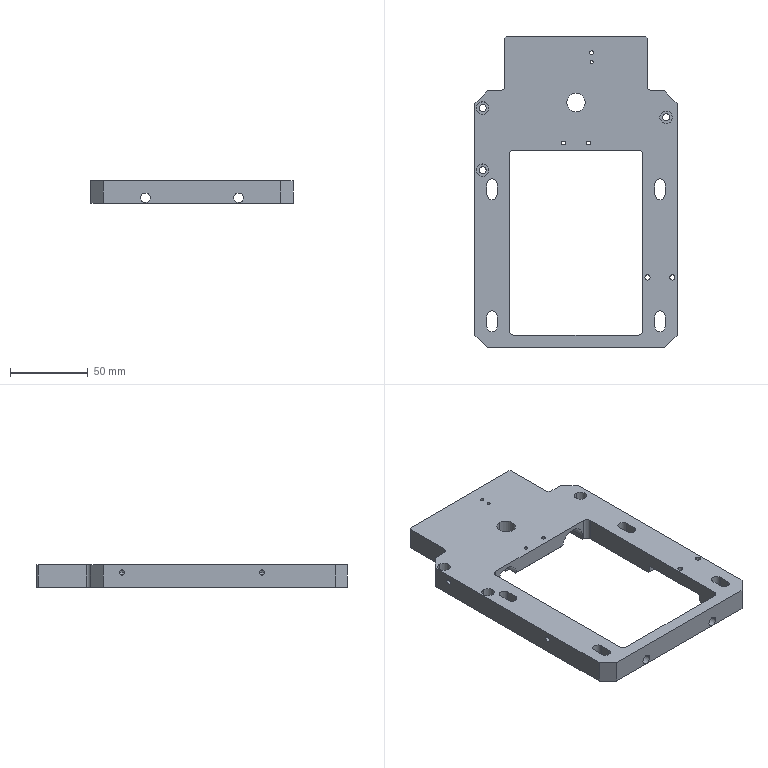NC program | NX | posted with a generic post | part box 130 x 200 x 14.5 mm
Lines 6565 to 7418 of 25347:
(ZLEVEL_PROFILE_1_COPY_1 , TOOL : D6)
N13062 T06 M6
N13064 G54
N13066 G17 G0 G90 X-88.086 Y-55.995 B0. C0. S4000 M3
N13068 G43 Z30. H6
N13070 Z1.5
N13072 G94 G1 X-88.016 Y-56.051 Z1.495 F1000.
N13074 X-87.513 Y-56.286 Z1.466
N13076 X-86.969 Y-56.4 Z1.437
N13078 X-79.531 Z1.047
N13080 X-79.017 Y-56.296 Z1.02
N13082 X-78.537 Y-56.083 Z0.992
N13084 X-78.115 Y-55.771 Z0.965
N13086 X-77.771 Y-55.375 Z0.937
N13088 X-77.52 Y-54.914 Z0.91
N13090 X-77.391 Y-54.495 Z0.887
N13092 X-77.341 Y-53.918 Z0.856
N13094 X-77.431 Y-53.346 Z0.826
N13096 X-77.654 Y-52.811 Z0.796
N13098 X-77.998 Y-52.345 Z0.765
N13100 X-78.443 Y-51.975 Z0.735
N13102 X-78.964 Y-51.722 Z0.705
N13104 X-79.531 Y-51.6 Z0.674
N13106 X-86.969 Z0.284
N13108 X-87.515 Y-51.715 Z0.255
N13110 X-88.019 Y-51.951 Z0.226
N13112 X-88.456 Y-52.298 Z0.197
N13114 X-88.801 Y-52.735 Z0.168
N13116 X-89.037 Y-53.24 Z0.138
N13118 X-89.15 Y-53.786 Z0.109
N13120 X-89.149 Y-54.225 Z0.086
N13122 X-89.034 Y-54.768 Z0.057
N13124 X-88.798 Y-55.271 Z0.028
N13126 X-88.452 Y-55.706 Z-0.001
N13128 X-88.016 Y-56.051 Z-0.03
N13130 X-87.513 Y-56.286 Z-0.059
N13132 X-86.969 Y-56.4 Z-0.089
N13134 X-86.75 Z-0.1
N13136 X-79.75 F1800.
N13138 G3 X-77.35 Y-54. R2.4
N13140 X-79.75 Y-51.6 R2.4
N13142 G1 X-86.75
N13144 G3 X-89.15 Y-54. R2.4
N13146 X-86.75 Y-56.4 R2.4
N13148 G1 X-82.538 Z-0.174
N13150 X-82.369 Y-56.399 Z-0.176
N13152 X-82.201 Y-56.4 Z-0.179
N13154 X-82.032 Y-56.399 Z-0.182
N13156 X-81.864 Y-56.4 Z-0.185
N13158 X-81.695 Y-56.399 Z-0.188
N13160 X-81.527 Y-56.4 Z-0.191
N13162 X-81.358 Y-56.399 Z-0.194
N13164 X-81.19 Y-56.4 Z-0.197
N13166 X-81.021 Z-0.2
N13168 X-79.75
N13170 G3 X-77.35 Y-54. R2.4
N13172 X-79.75 Y-51.6 R2.4
N13174 G1 X-86.75
N13176 G3 X-89.15 Y-54. R2.4
N13178 X-86.75 Y-56.4 R2.4
N13180 G1 X-82.538 Z-0.274
N13182 X-82.369 Y-56.399 Z-0.276
N13184 X-82.201 Y-56.4 Z-0.279
N13186 X-82.032 Y-56.399 Z-0.282
N13188 X-81.864 Y-56.4 Z-0.285
N13190 X-81.695 Y-56.399 Z-0.288
N13192 X-81.527 Y-56.4 Z-0.291
N13194 X-81.358 Y-56.399 Z-0.294
N13196 X-81.19 Y-56.4 Z-0.297
N13198 X-81.021 Z-0.3
N13200 X-79.75
N13202 G3 X-77.35 Y-54. R2.4
N13204 X-79.75 Y-51.6 R2.4
N13206 G1 X-86.75
N13208 G3 X-89.15 Y-54. R2.4
N13210 X-86.75 Y-56.4 R2.4
N13212 G1 X-82.538 Z-0.374
N13214 X-82.369 Y-56.399 Z-0.376
N13216 X-82.201 Y-56.4 Z-0.379
N13218 X-82.032 Y-56.399 Z-0.382
N13220 X-81.864 Y-56.4 Z-0.385
N13222 X-81.695 Y-56.399 Z-0.388
N13224 X-81.527 Y-56.4 Z-0.391
N13226 X-81.358 Y-56.399 Z-0.394
N13228 X-81.19 Y-56.4 Z-0.397
N13230 X-81.021 Z-0.4
N13232 X-79.75
N13234 G3 X-77.35 Y-54. R2.4
N13236 X-79.75 Y-51.6 R2.4
N13238 G1 X-86.75
N13240 G3 X-89.15 Y-54. R2.4
N13242 X-86.75 Y-56.4 R2.4
N13244 G1 X-82.538 Z-0.474
N13246 X-82.369 Y-56.399 Z-0.476
N13248 X-82.201 Y-56.4 Z-0.479
N13250 X-82.032 Y-56.399 Z-0.482
N13252 X-81.864 Y-56.4 Z-0.485
N13254 X-81.695 Y-56.399 Z-0.488
N13256 X-81.527 Y-56.4 Z-0.491
N13258 X-81.358 Y-56.399 Z-0.494
N13260 X-81.19 Y-56.4 Z-0.497
N13262 X-81.021 Z-0.5
N13264 X-79.75
N13266 G3 X-77.35 Y-54. R2.4
N13268 X-79.75 Y-51.6 R2.4
N13270 G1 X-86.75
N13272 G3 X-89.15 Y-54. R2.4
N13274 X-86.75 Y-56.4 R2.4
N13276 G1 X-82.538 Z-0.574
N13278 X-82.369 Y-56.399 Z-0.576
N13280 X-82.201 Y-56.4 Z-0.579
N13282 X-82.032 Y-56.399 Z-0.582
N13284 X-81.864 Y-56.4 Z-0.585
N13286 X-81.695 Y-56.399 Z-0.588
N13288 X-81.527 Y-56.4 Z-0.591
N13290 X-81.358 Y-56.399 Z-0.594
N13292 X-81.19 Y-56.4 Z-0.597
N13294 X-81.021 Z-0.6
N13296 X-79.75
N13298 G3 X-77.35 Y-54. R2.4
N13300 X-79.75 Y-51.6 R2.4
N13302 G1 X-86.75
N13304 G3 X-89.15 Y-54. R2.4
N13306 X-86.75 Y-56.4 R2.4
N13308 G1 X-82.538 Z-0.674
N13310 X-82.369 Y-56.399 Z-0.676
N13312 X-82.201 Y-56.4 Z-0.679
N13314 X-82.032 Y-56.399 Z-0.682
N13316 X-81.864 Y-56.4 Z-0.685
N13318 X-81.695 Y-56.399 Z-0.688
N13320 X-81.527 Y-56.4 Z-0.691
N13322 X-81.358 Y-56.399 Z-0.694
N13324 X-81.19 Y-56.4 Z-0.697
N13326 X-81.021 Z-0.7
N13328 X-79.75
N13330 G3 X-77.35 Y-54. R2.4
N13332 X-79.75 Y-51.6 R2.4
N13334 G1 X-86.75
N13336 G3 X-89.15 Y-54. R2.4
N13338 X-86.75 Y-56.4 R2.4
N13340 G1 X-82.538 Z-0.774
N13342 X-82.369 Y-56.399 Z-0.776
N13344 X-82.201 Y-56.4 Z-0.779
N13346 X-82.032 Y-56.399 Z-0.782
N13348 X-81.864 Y-56.4 Z-0.785
N13350 X-81.695 Y-56.399 Z-0.788
N13352 X-81.527 Y-56.4 Z-0.791
N13354 X-81.358 Y-56.399 Z-0.794
N13356 X-81.19 Y-56.4 Z-0.797
N13358 X-81.021 Z-0.8
N13360 X-79.75
N13362 G3 X-77.35 Y-54. R2.4
N13364 X-79.75 Y-51.6 R2.4
N13366 G1 X-86.75
N13368 G3 X-89.15 Y-54. R2.4
N13370 X-86.75 Y-56.4 R2.4
N13372 G1 X-82.538 Z-0.874
N13374 X-82.369 Y-56.399 Z-0.876
N13376 X-82.201 Y-56.4 Z-0.879
N13378 X-82.032 Y-56.399 Z-0.882
N13380 X-81.864 Y-56.4 Z-0.885
N13382 X-81.695 Y-56.399 Z-0.888
N13384 X-81.527 Y-56.4 Z-0.891
N13386 X-81.358 Y-56.399 Z-0.894
N13388 X-81.19 Y-56.4 Z-0.897
N13390 X-81.021 Z-0.9
N13392 X-79.75
N13394 G3 X-77.35 Y-54. R2.4
N13396 X-79.75 Y-51.6 R2.4
N13398 G1 X-86.75
N13400 G3 X-89.15 Y-54. R2.4
N13402 X-86.75 Y-56.4 R2.4
N13404 G1 X-82.538 Z-0.974
N13406 X-82.369 Y-56.399 Z-0.976
N13408 X-82.201 Y-56.4 Z-0.979
N13410 X-82.032 Y-56.399 Z-0.982
N13412 X-81.864 Y-56.4 Z-0.985
N13414 X-81.695 Y-56.399 Z-0.988
N13416 X-81.527 Y-56.4 Z-0.991
N13418 X-81.358 Y-56.399 Z-0.994
N13420 X-81.19 Y-56.4 Z-0.997
N13422 X-81.021 Z-1.
N13424 X-79.75
N13426 G3 X-77.35 Y-54. R2.4
N13428 X-79.75 Y-51.6 R2.4
N13430 G1 X-86.75
N13432 G3 X-89.15 Y-54. R2.4
N13434 X-86.75 Y-56.4 R2.4
N13436 G1 X-82.538 Z-1.074
N13438 X-82.369 Y-56.399 Z-1.076
N13440 X-82.201 Y-56.4 Z-1.079
N13442 X-82.032 Y-56.399 Z-1.082
N13444 X-81.864 Y-56.4 Z-1.085
N13446 X-81.695 Y-56.399 Z-1.088
N13448 X-81.527 Y-56.4 Z-1.091
N13450 X-81.358 Y-56.399 Z-1.094
N13452 X-81.19 Y-56.4 Z-1.097
N13454 X-81.021 Z-1.1
N13456 X-79.75
N13458 G3 X-77.35 Y-54. R2.4
N13460 X-79.75 Y-51.6 R2.4
N13462 G1 X-86.75
N13464 G3 X-89.15 Y-54. R2.4
N13466 X-86.75 Y-56.4 R2.4
N13468 G1 X-82.538 Z-1.174
N13470 X-82.369 Y-56.399 Z-1.176
N13472 X-82.201 Y-56.4 Z-1.179
N13474 X-82.032 Y-56.399 Z-1.182
N13476 X-81.864 Y-56.4 Z-1.185
N13478 X-81.695 Y-56.399 Z-1.188
N13480 X-81.527 Y-56.4 Z-1.191
N13482 X-81.358 Y-56.399 Z-1.194
N13484 X-81.19 Y-56.4 Z-1.197
N13486 X-81.021 Z-1.2
N13488 X-79.75
N13490 G3 X-77.35 Y-54. R2.4
N13492 X-79.75 Y-51.6 R2.4
N13494 G1 X-86.75
N13496 G3 X-89.15 Y-54. R2.4
N13498 X-86.75 Y-56.4 R2.4
N13500 G1 X-82.538 Z-1.274
N13502 X-82.369 Y-56.399 Z-1.276
N13504 X-82.201 Y-56.4 Z-1.279
N13506 X-82.032 Y-56.399 Z-1.282
N13508 X-81.864 Y-56.4 Z-1.285
N13510 X-81.695 Y-56.399 Z-1.288
N13512 X-81.527 Y-56.4 Z-1.291
N13514 X-81.358 Y-56.399 Z-1.294
N13516 X-81.19 Y-56.4 Z-1.297
N13518 X-81.021 Z-1.3
N13520 X-79.75
N13522 G3 X-77.35 Y-54. R2.4
N13524 X-79.75 Y-51.6 R2.4
N13526 G1 X-86.75
N13528 G3 X-89.15 Y-54. R2.4
N13530 X-86.75 Y-56.4 R2.4
N13532 G1 X-82.538 Z-1.374
N13534 X-82.369 Y-56.399 Z-1.376
N13536 X-82.201 Y-56.4 Z-1.379
N13538 X-82.032 Y-56.399 Z-1.382
N13540 X-81.864 Y-56.4 Z-1.385
N13542 X-81.695 Y-56.399 Z-1.388
N13544 X-81.527 Y-56.4 Z-1.391
N13546 X-81.358 Y-56.399 Z-1.394
N13548 X-81.19 Y-56.4 Z-1.397
N13550 X-81.021 Z-1.4
N13552 X-79.75
N13554 G3 X-77.35 Y-54. R2.4
N13556 X-79.75 Y-51.6 R2.4
N13558 G1 X-86.75
N13560 G3 X-89.15 Y-54. R2.4
N13562 X-86.75 Y-56.4 R2.4
N13564 G1 X-82.538 Z-1.474
N13566 X-82.369 Y-56.399 Z-1.476
N13568 X-82.201 Y-56.4 Z-1.479
N13570 X-82.032 Y-56.399 Z-1.482
N13572 X-81.864 Y-56.4 Z-1.485
N13574 X-81.695 Y-56.399 Z-1.488
N13576 X-81.527 Y-56.4 Z-1.491
N13578 X-81.358 Y-56.399 Z-1.494
N13580 X-81.19 Y-56.4 Z-1.497
N13582 X-81.021 Z-1.5
N13584 X-79.75
N13586 G3 X-77.35 Y-54. R2.4
N13588 X-79.75 Y-51.6 R2.4
N13590 G1 X-86.75
N13592 G3 X-89.15 Y-54. R2.4
N13594 X-86.75 Y-56.4 R2.4
N13596 G1 X-82.538 Z-1.574
N13598 X-82.369 Y-56.399 Z-1.576
N13600 X-82.201 Y-56.4 Z-1.579
N13602 X-82.032 Y-56.399 Z-1.582
N13604 X-81.864 Y-56.4 Z-1.585
N13606 X-81.695 Y-56.399 Z-1.588
N13608 X-81.527 Y-56.4 Z-1.591
N13610 X-81.358 Y-56.399 Z-1.594
N13612 X-81.19 Y-56.4 Z-1.597
N13614 X-81.021 Z-1.6
N13616 X-79.75
N13618 G3 X-77.35 Y-54. R2.4
N13620 X-79.75 Y-51.6 R2.4
N13622 G1 X-86.75
N13624 G3 X-89.15 Y-54. R2.4
N13626 X-86.75 Y-56.4 R2.4
N13628 G1 X-82.538 Z-1.674
N13630 X-82.369 Y-56.399 Z-1.676
N13632 X-82.201 Y-56.4 Z-1.679
N13634 X-82.032 Y-56.399 Z-1.682
N13636 X-81.864 Y-56.4 Z-1.685
N13638 X-81.695 Y-56.399 Z-1.688
N13640 X-81.527 Y-56.4 Z-1.691
N13642 X-81.358 Y-56.399 Z-1.694
N13644 X-81.19 Y-56.4 Z-1.697
N13646 X-81.021 Z-1.7
N13648 X-79.75
N13650 G3 X-77.35 Y-54. R2.4
N13652 X-79.75 Y-51.6 R2.4
N13654 G1 X-86.75
N13656 G3 X-89.15 Y-54. R2.4
N13658 X-86.75 Y-56.4 R2.4
N13660 G1 X-82.538 Z-1.774
N13662 X-82.369 Y-56.399 Z-1.776
N13664 X-82.201 Y-56.4 Z-1.779
N13666 X-82.032 Y-56.399 Z-1.782
N13668 X-81.864 Y-56.4 Z-1.785
N13670 X-81.695 Y-56.399 Z-1.788
N13672 X-81.527 Y-56.4 Z-1.791
N13674 X-81.358 Y-56.399 Z-1.794
N13676 X-81.19 Y-56.4 Z-1.797
N13678 X-81.021 Z-1.8
N13680 X-79.75
N13682 G3 X-77.35 Y-54. R2.4
N13684 X-79.75 Y-51.6 R2.4
N13686 G1 X-86.75
N13688 G3 X-89.15 Y-54. R2.4
N13690 X-86.75 Y-56.4 R2.4
N13692 G1 X-82.538 Z-1.874
N13694 X-82.369 Y-56.399 Z-1.876
N13696 X-82.201 Y-56.4 Z-1.879
N13698 X-82.032 Y-56.399 Z-1.882
N13700 X-81.864 Y-56.4 Z-1.885
N13702 X-81.695 Y-56.399 Z-1.888
N13704 X-81.527 Y-56.4 Z-1.891
N13706 X-81.358 Y-56.399 Z-1.894
N13708 X-81.19 Y-56.4 Z-1.897
N13710 X-81.021 Z-1.9
N13712 X-79.75
N13714 G3 X-77.35 Y-54. R2.4
N13716 X-79.75 Y-51.6 R2.4
N13718 G1 X-86.75
N13720 G3 X-89.15 Y-54. R2.4
N13722 X-86.75 Y-56.4 R2.4
N13724 G1 X-82.538 Z-1.974
N13726 X-82.369 Y-56.399 Z-1.976
N13728 X-82.201 Y-56.4 Z-1.979
N13730 X-82.032 Y-56.399 Z-1.982
N13732 X-81.864 Y-56.4 Z-1.985
N13734 X-81.695 Y-56.399 Z-1.988
N13736 X-81.527 Y-56.4 Z-1.991
N13738 X-81.358 Y-56.399 Z-1.994
N13740 X-81.19 Y-56.4 Z-1.997
N13742 X-81.021 Z-2.
N13744 X-79.75
N13746 G3 X-77.35 Y-54. R2.4
N13748 X-79.75 Y-51.6 R2.4
N13750 G1 X-86.75
N13752 G3 X-89.15 Y-54. R2.4
N13754 X-86.75 Y-56.4 R2.4
N13756 G1 X-82.538 Z-2.074
N13758 X-82.369 Y-56.399 Z-2.076
N13760 X-82.201 Y-56.4 Z-2.079
N13762 X-82.032 Y-56.399 Z-2.082
N13764 X-81.864 Y-56.4 Z-2.085
N13766 X-81.695 Y-56.399 Z-2.088
N13768 X-81.527 Y-56.4 Z-2.091
N13770 X-81.358 Y-56.399 Z-2.094
N13772 X-81.19 Y-56.4 Z-2.097
N13774 X-81.021 Z-2.1
N13776 X-79.75
N13778 G3 X-77.35 Y-54. R2.4
N13780 X-79.75 Y-51.6 R2.4
N13782 G1 X-86.75
N13784 G3 X-89.15 Y-54. R2.4
N13786 X-86.75 Y-56.4 R2.4
N13788 G1 X-82.538 Z-2.174
N13790 X-82.369 Y-56.399 Z-2.176
N13792 X-82.201 Y-56.4 Z-2.179
N13794 X-82.032 Y-56.399 Z-2.182
N13796 X-81.864 Y-56.4 Z-2.185
N13798 X-81.695 Y-56.399 Z-2.188
N13800 X-81.527 Y-56.4 Z-2.191
N13802 X-81.358 Y-56.399 Z-2.194
N13804 X-81.19 Y-56.4 Z-2.197
N13806 X-81.021 Z-2.2
N13808 X-79.75
N13810 G3 X-77.35 Y-54. R2.4
N13812 X-79.75 Y-51.6 R2.4
N13814 G1 X-86.75
N13816 G3 X-89.15 Y-54. R2.4
N13818 X-86.75 Y-56.4 R2.4
N13820 G1 X-82.538 Z-2.274
N13822 X-82.369 Y-56.399 Z-2.276
N13824 X-82.201 Y-56.4 Z-2.279
N13826 X-82.032 Y-56.399 Z-2.282
N13828 X-81.864 Y-56.4 Z-2.285
N13830 X-81.695 Y-56.399 Z-2.288
N13832 X-81.527 Y-56.4 Z-2.291
N13834 X-81.358 Y-56.399 Z-2.294
N13836 X-81.19 Y-56.4 Z-2.297
N13838 X-81.021 Z-2.3
N13840 X-79.75
N13842 G3 X-77.35 Y-54. R2.4
N13844 X-79.75 Y-51.6 R2.4
N13846 G1 X-86.75
N13848 G3 X-89.15 Y-54. R2.4
N13850 X-86.75 Y-56.4 R2.4
N13852 G1 X-82.538 Z-2.374
N13854 X-82.369 Y-56.399 Z-2.376
N13856 X-82.201 Y-56.4 Z-2.379
N13858 X-82.032 Y-56.399 Z-2.382
N13860 X-81.864 Y-56.4 Z-2.385
N13862 X-81.695 Y-56.399 Z-2.388
N13864 X-81.527 Y-56.4 Z-2.391
N13866 X-81.358 Y-56.399 Z-2.394
N13868 X-81.19 Y-56.4 Z-2.397
N13870 X-81.021 Z-2.4
N13872 X-79.75
N13874 G3 X-77.35 Y-54. R2.4
N13876 X-79.75 Y-51.6 R2.4
N13878 G1 X-86.75
N13880 G3 X-89.15 Y-54. R2.4
N13882 X-86.75 Y-56.4 R2.4
N13884 G1 X-82.538 Z-2.474
N13886 X-82.369 Y-56.399 Z-2.476
N13888 X-82.201 Y-56.4 Z-2.479
N13890 X-82.032 Y-56.399 Z-2.482
N13892 X-81.864 Y-56.4 Z-2.485
N13894 X-81.695 Y-56.399 Z-2.488
N13896 X-81.527 Y-56.4 Z-2.491
N13898 X-81.358 Y-56.399 Z-2.494
N13900 X-81.19 Y-56.4 Z-2.497
N13902 X-81.021 Z-2.5
N13904 X-79.75
N13906 G3 X-77.35 Y-54. R2.4
N13908 X-79.75 Y-51.6 R2.4
N13910 G1 X-86.75
N13912 G3 X-89.15 Y-54. R2.4
N13914 X-86.75 Y-56.4 R2.4
N13916 G1 X-82.538 Z-2.574
N13918 X-82.369 Y-56.399 Z-2.576
N13920 X-82.201 Y-56.4 Z-2.579
N13922 X-82.032 Y-56.399 Z-2.582
N13924 X-81.864 Y-56.4 Z-2.585
N13926 X-81.695 Y-56.399 Z-2.588
N13928 X-81.527 Y-56.4 Z-2.591
N13930 X-81.358 Y-56.399 Z-2.594
N13932 X-81.19 Y-56.4 Z-2.597
N13934 X-81.021 Z-2.6
N13936 X-79.75
N13938 G3 X-77.35 Y-54. R2.4
N13940 X-79.75 Y-51.6 R2.4
N13942 G1 X-86.75
N13944 G3 X-89.15 Y-54. R2.4
N13946 X-86.75 Y-56.4 R2.4
N13948 G1 X-82.538 Z-2.674
N13950 X-82.369 Y-56.399 Z-2.676
N13952 X-82.201 Y-56.4 Z-2.679
N13954 X-82.032 Y-56.399 Z-2.682
N13956 X-81.864 Y-56.4 Z-2.685
N13958 X-81.695 Y-56.399 Z-2.688
N13960 X-81.527 Y-56.4 Z-2.691
N13962 X-81.358 Y-56.399 Z-2.694
N13964 X-81.19 Y-56.4 Z-2.697
N13966 X-81.021 Z-2.7
N13968 X-79.75
N13970 G3 X-77.35 Y-54. R2.4
N13972 X-79.75 Y-51.6 R2.4
N13974 G1 X-86.75
N13976 G3 X-89.15 Y-54. R2.4
N13978 X-86.75 Y-56.4 R2.4
N13980 G1 X-82.538 Z-2.774
N13982 X-82.369 Y-56.399 Z-2.776
N13984 X-82.201 Y-56.4 Z-2.779
N13986 X-82.032 Y-56.399 Z-2.782
N13988 X-81.864 Y-56.4 Z-2.785
N13990 X-81.695 Y-56.399 Z-2.788
N13992 X-81.527 Y-56.4 Z-2.791
N13994 X-81.358 Y-56.399 Z-2.794
N13996 X-81.19 Y-56.4 Z-2.797
N13998 X-81.021 Z-2.8
N14000 X-79.75
N14002 G3 X-77.35 Y-54. R2.4
N14004 X-79.75 Y-51.6 R2.4
N14006 G1 X-86.75
N14008 G3 X-89.15 Y-54. R2.4
N14010 X-86.75 Y-56.4 R2.4
N14012 G1 X-82.538 Z-2.874
N14014 X-82.369 Y-56.399 Z-2.876
N14016 X-82.201 Y-56.4 Z-2.879
N14018 X-82.032 Y-56.399 Z-2.882
N14020 X-81.864 Y-56.4 Z-2.885
N14022 X-81.695 Y-56.399 Z-2.888
N14024 X-81.527 Y-56.4 Z-2.891
N14026 X-81.358 Y-56.399 Z-2.894
N14028 X-81.19 Y-56.4 Z-2.897
N14030 X-81.021 Z-2.9
N14032 X-79.75
N14034 G3 X-77.35 Y-54. R2.4
N14036 X-79.75 Y-51.6 R2.4
N14038 G1 X-86.75
N14040 G3 X-89.15 Y-54. R2.4
N14042 X-86.75 Y-56.4 R2.4
N14044 G1 X-82.538 Z-2.974
N14046 X-82.369 Y-56.399 Z-2.976
N14048 X-82.201 Y-56.4 Z-2.979
N14050 X-82.032 Y-56.399 Z-2.982
N14052 X-81.864 Y-56.4 Z-2.985
N14054 X-81.695 Y-56.399 Z-2.988
N14056 X-81.527 Y-56.4 Z-2.991
N14058 X-81.358 Y-56.399 Z-2.994
N14060 X-81.19 Y-56.4 Z-2.997
N14062 X-81.021 Z-3.
N14064 X-79.75
N14066 G3 X-77.35 Y-54. R2.4
N14068 X-79.75 Y-51.6 R2.4
N14070 G1 X-86.75
N14072 G3 X-89.15 Y-54. R2.4
N14074 X-86.75 Y-56.4 R2.4
N14076 G1 X-82.538 Z-3.074
N14078 X-82.369 Y-56.399 Z-3.076
N14080 X-82.201 Y-56.4 Z-3.079
N14082 X-82.032 Y-56.399 Z-3.082
N14084 X-81.864 Y-56.4 Z-3.085
N14086 X-81.695 Y-56.399 Z-3.088
N14088 X-81.527 Y-56.4 Z-3.091
N14090 X-81.358 Y-56.399 Z-3.094
N14092 X-81.19 Y-56.4 Z-3.097
N14094 X-81.021 Z-3.1
N14096 X-79.75
N14098 G3 X-77.35 Y-54. R2.4
N14100 X-79.75 Y-51.6 R2.4
N14102 G1 X-86.75
N14104 G3 X-89.15 Y-54. R2.4
N14106 X-86.75 Y-56.4 R2.4
N14108 G1 X-82.538 Z-3.174
N14110 X-82.369 Y-56.399 Z-3.176
N14112 X-82.201 Y-56.4 Z-3.179
N14114 X-82.032 Y-56.399 Z-3.182
N14116 X-81.864 Y-56.4 Z-3.185
N14118 X-81.695 Y-56.399 Z-3.188
N14120 X-81.527 Y-56.4 Z-3.191
N14122 X-81.358 Y-56.399 Z-3.194
N14124 X-81.19 Y-56.4 Z-3.197
N14126 X-81.021 Z-3.2
N14128 X-79.75
N14130 G3 X-77.35 Y-54. R2.4
N14132 X-79.75 Y-51.6 R2.4
N14134 G1 X-86.75
N14136 G3 X-89.15 Y-54. R2.4
N14138 X-86.75 Y-56.4 R2.4
N14140 G1 X-82.538 Z-3.274
N14142 X-82.369 Y-56.399 Z-3.276
N14144 X-82.201 Y-56.4 Z-3.279
N14146 X-82.032 Y-56.399 Z-3.282
N14148 X-81.864 Y-56.4 Z-3.285
N14150 X-81.695 Y-56.399 Z-3.288
N14152 X-81.527 Y-56.4 Z-3.291
N14154 X-81.358 Y-56.399 Z-3.294
N14156 X-81.19 Y-56.4 Z-3.297
N14158 X-81.021 Z-3.3
N14160 X-79.75
N14162 G3 X-77.35 Y-54. R2.4
N14164 X-79.75 Y-51.6 R2.4
N14166 G1 X-86.75
N14168 G3 X-89.15 Y-54. R2.4
N14170 X-86.75 Y-56.4 R2.4
N14172 G1 X-82.538 Z-3.374
N14174 X-82.369 Y-56.399 Z-3.376
N14176 X-82.201 Y-56.4 Z-3.379
N14178 X-82.032 Y-56.399 Z-3.382
N14180 X-81.864 Y-56.4 Z-3.385
N14182 X-81.695 Y-56.399 Z-3.388
N14184 X-81.527 Y-56.4 Z-3.391
N14186 X-81.358 Y-56.399 Z-3.394
N14188 X-81.19 Y-56.4 Z-3.397
N14190 X-81.021 Z-3.4
N14192 X-79.75
N14194 G3 X-77.35 Y-54. R2.4
N14196 X-79.75 Y-51.6 R2.4
N14198 G1 X-86.75
N14200 G3 X-89.15 Y-54. R2.4
N14202 X-86.75 Y-56.4 R2.4
N14204 G1 X-82.538 Z-3.474
N14206 X-82.369 Y-56.399 Z-3.476
N14208 X-82.201 Y-56.4 Z-3.479
N14210 X-82.032 Y-56.399 Z-3.482
N14212 X-81.864 Y-56.4 Z-3.485
N14214 X-81.695 Y-56.399 Z-3.488
N14216 X-81.527 Y-56.4 Z-3.491
N14218 X-81.358 Y-56.399 Z-3.494
N14220 X-81.19 Y-56.4 Z-3.497
N14222 X-81.021 Z-3.5
N14224 X-79.75
N14226 G3 X-77.35 Y-54. R2.4
N14228 X-79.75 Y-51.6 R2.4
N14230 G1 X-86.75
N14232 G3 X-89.15 Y-54. R2.4
N14234 X-86.75 Y-56.4 R2.4
N14236 G1 X-82.538 Z-3.574
N14238 X-82.369 Y-56.399 Z-3.576
N14240 X-82.201 Y-56.4 Z-3.579
N14242 X-82.032 Y-56.399 Z-3.582
N14244 X-81.864 Y-56.4 Z-3.585
N14246 X-81.695 Y-56.399 Z-3.588
N14248 X-81.527 Y-56.4 Z-3.591
N14250 X-81.358 Y-56.399 Z-3.594
N14252 X-81.19 Y-56.4 Z-3.597
N14254 X-81.021 Z-3.6
N14256 X-79.75
N14258 G3 X-77.35 Y-54. R2.4
N14260 X-79.75 Y-51.6 R2.4
N14262 G1 X-86.75
N14264 G3 X-89.15 Y-54. R2.4
N14266 X-86.75 Y-56.4 R2.4
N14268 G1 X-82.538 Z-3.674
N14270 X-82.369 Y-56.399 Z-3.676
N14272 X-82.201 Y-56.4 Z-3.679
N14274 X-82.032 Y-56.399 Z-3.682
N14276 X-81.864 Y-56.4 Z-3.685
N14278 X-81.695 Y-56.399 Z-3.688
N14280 X-81.527 Y-56.4 Z-3.691
N14282 X-81.358 Y-56.399 Z-3.694
N14284 X-81.19 Y-56.4 Z-3.697
N14286 X-81.021 Z-3.7
N14288 X-79.75
N14290 G3 X-77.35 Y-54. R2.4
N14292 X-79.75 Y-51.6 R2.4
N14294 G1 X-86.75
N14296 G3 X-89.15 Y-54. R2.4
N14298 X-86.75 Y-56.4 R2.4
N14300 G1 X-82.538 Z-3.774
N14302 X-82.369 Y-56.399 Z-3.776
N14304 X-82.201 Y-56.4 Z-3.779
N14306 X-82.032 Y-56.399 Z-3.782
N14308 X-81.864 Y-56.4 Z-3.785
N14310 X-81.695 Y-56.399 Z-3.788
N14312 X-81.527 Y-56.4 Z-3.791
N14314 X-81.358 Y-56.399 Z-3.794
N14316 X-81.19 Y-56.4 Z-3.797
N14318 X-81.021 Z-3.8
N14320 X-79.75
N14322 G3 X-77.35 Y-54. R2.4
N14324 X-79.75 Y-51.6 R2.4
N14326 G1 X-86.75
N14328 G3 X-89.15 Y-54. R2.4
N14330 X-86.75 Y-56.4 R2.4
N14332 G1 X-82.538 Z-3.874
N14334 X-82.369 Y-56.399 Z-3.876
N14336 X-82.201 Y-56.4 Z-3.879
N14338 X-82.032 Y-56.399 Z-3.882
N14340 X-81.864 Y-56.4 Z-3.885
N14342 X-81.695 Y-56.399 Z-3.888
N14344 X-81.527 Y-56.4 Z-3.891
N14346 X-81.358 Y-56.399 Z-3.894
N14348 X-81.19 Y-56.4 Z-3.897
N14350 X-81.021 Z-3.9
N14352 X-79.75
N14354 G3 X-77.35 Y-54. R2.4
N14356 X-79.75 Y-51.6 R2.4
N14358 G1 X-86.75
N14360 G3 X-89.15 Y-54. R2.4
N14362 X-86.75 Y-56.4 R2.4
N14364 G1 X-82.538 Z-3.974
N14366 X-82.369 Y-56.399 Z-3.976
N14368 X-82.201 Y-56.4 Z-3.979
N14370 X-82.032 Y-56.399 Z-3.982
N14372 X-81.864 Y-56.4 Z-3.985
N14374 X-81.695 Y-56.399 Z-3.988
N14376 X-81.527 Y-56.4 Z-3.991
N14378 X-81.358 Y-56.399 Z-3.994
N14380 X-81.19 Y-56.4 Z-3.997
N14382 X-81.021 Z-4.
N14384 X-79.75
N14386 G3 X-77.35 Y-54. R2.4
N14388 X-79.75 Y-51.6 R2.4
N14390 G1 X-86.75
N14392 G3 X-89.15 Y-54. R2.4
N14394 X-86.75 Y-56.4 R2.4
N14396 G1 X-82.538 Z-4.074
N14398 X-82.369 Y-56.399 Z-4.076
N14400 X-82.201 Y-56.4 Z-4.079
N14402 X-82.032 Y-56.399 Z-4.082
N14404 X-81.864 Y-56.4 Z-4.085
N14406 X-81.695 Y-56.399 Z-4.088
N14408 X-81.527 Y-56.4 Z-4.091
N14410 X-81.358 Y-56.399 Z-4.094
N14412 X-81.19 Y-56.4 Z-4.097
N14414 X-81.021 Z-4.1
N14416 X-79.75
N14418 G3 X-77.35 Y-54. R2.4
N14420 X-79.75 Y-51.6 R2.4
N14422 G1 X-86.75
N14424 G3 X-89.15 Y-54. R2.4
N14426 X-86.75 Y-56.4 R2.4
N14428 G1 X-82.538 Z-4.174
N14430 X-82.369 Y-56.398 Z-4.176
N14432 X-82.201 Y-56.4 Z-4.179
N14434 X-82.032 Y-56.398 Z-4.182
N14436 X-81.864 Y-56.4 Z-4.185
N14438 X-81.695 Y-56.398 Z-4.188
N14440 X-81.527 Y-56.4 Z-4.191
N14442 X-81.358 Y-56.398 Z-4.194
N14444 X-81.19 Y-56.4 Z-4.197
N14446 X-81.021 Z-4.2
N14448 X-79.75
N14450 G3 X-77.35 Y-54. R2.4
N14452 X-79.75 Y-51.6 R2.4
N14454 G1 X-86.75
N14456 G3 X-89.15 Y-54. R2.4
N14458 X-86.75 Y-56.4 R2.4
N14460 G1 X-82.538 Z-4.274
N14462 X-82.369 Y-56.398 Z-4.276
N14464 X-82.201 Y-56.4 Z-4.279
N14466 X-82.032 Y-56.398 Z-4.282
N14468 X-81.864 Y-56.4 Z-4.285
N14470 X-81.695 Y-56.398 Z-4.288
N14472 X-81.527 Y-56.4 Z-4.291
N14474 X-81.358 Y-56.398 Z-4.294
N14476 X-81.19 Y-56.4 Z-4.297
N14478 X-81.021 Z-4.3
N14480 X-79.75
N14482 G3 X-77.35 Y-54. R2.4
N14484 X-79.75 Y-51.6 R2.4
N14486 G1 X-86.75
N14488 G3 X-89.15 Y-54. R2.4
N14490 X-86.75 Y-56.4 R2.4
N14492 G1 X-82.538 Z-4.374
N14494 X-82.369 Y-56.398 Z-4.376
N14496 X-82.201 Y-56.4 Z-4.379
N14498 X-82.032 Y-56.398 Z-4.382
N14500 X-81.864 Y-56.4 Z-4.385
N14502 X-81.695 Y-56.398 Z-4.388
N14504 X-81.527 Y-56.4 Z-4.391
N14506 X-81.358 Y-56.398 Z-4.394
N14508 X-81.19 Y-56.4 Z-4.397
N14510 X-81.021 Z-4.4
N14512 X-79.75
N14514 G3 X-77.35 Y-54. R2.4
N14516 X-79.75 Y-51.6 R2.4
N14518 G1 X-86.75
N14520 G3 X-89.15 Y-54. R2.4
N14522 X-86.75 Y-56.4 R2.4
N14524 G1 X-82.538 Z-4.474
N14526 X-82.369 Y-56.398 Z-4.476
N14528 X-82.201 Y-56.4 Z-4.479
N14530 X-82.032 Y-56.398 Z-4.482
N14532 X-81.864 Y-56.4 Z-4.485
N14534 X-81.695 Y-56.398 Z-4.488
N14536 X-81.527 Y-56.4 Z-4.491
N14538 X-81.358 Y-56.398 Z-4.494
N14540 X-81.19 Y-56.4 Z-4.497
N14542 X-81.021 Z-4.5
N14544 X-79.75
N14546 G3 X-77.35 Y-54. R2.4
N14548 X-79.75 Y-51.6 R2.4
N14550 G1 X-86.75
N14552 G3 X-89.15 Y-54. R2.4
N14554 X-86.75 Y-56.4 R2.4
N14556 G1 X-82.538 Z-4.574
N14558 X-82.369 Y-56.398 Z-4.576
N14560 X-82.201 Y-56.4 Z-4.579
N14562 X-82.032 Y-56.398 Z-4.582
N14564 X-81.864 Y-56.4 Z-4.585
N14566 X-81.695 Y-56.398 Z-4.588
N14568 X-81.527 Y-56.4 Z-4.591
N14570 X-81.358 Y-56.398 Z-4.594
N14572 X-81.19 Y-56.4 Z-4.597
N14574 X-81.021 Z-4.6
N14576 X-79.75
N14578 G3 X-77.35 Y-54. R2.4
N14580 X-79.75 Y-51.6 R2.4
N14582 G1 X-86.75
N14584 G3 X-89.15 Y-54. R2.4
N14586 X-86.75 Y-56.4 R2.4
N14588 G1 X-82.538 Z-4.674
N14590 X-82.369 Y-56.398 Z-4.676
N14592 X-82.201 Y-56.4 Z-4.679
N14594 X-82.032 Y-56.398 Z-4.682
N14596 X-81.864 Y-56.4 Z-4.685
N14598 X-81.695 Y-56.398 Z-4.688
N14600 X-81.527 Y-56.4 Z-4.691
N14602 X-81.358 Y-56.398 Z-4.694
N14604 X-81.19 Y-56.4 Z-4.697
N14606 X-81.021 Z-4.7
N14608 X-79.75
N14610 G3 X-77.35 Y-54. R2.4
N14612 X-79.75 Y-51.6 R2.4
N14614 G1 X-86.75
N14616 G3 X-89.15 Y-54. R2.4
N14618 X-86.75 Y-56.4 R2.4
N14620 G1 X-82.538 Z-4.774
N14622 X-82.369 Y-56.398 Z-4.776
N14624 X-82.201 Y-56.4 Z-4.779
N14626 X-82.032 Y-56.398 Z-4.782
N14628 X-81.864 Y-56.4 Z-4.785
N14630 X-81.695 Y-56.398 Z-4.788
N14632 X-81.527 Y-56.4 Z-4.791
N14634 X-81.358 Y-56.398 Z-4.794
N14636 X-81.19 Y-56.4 Z-4.797
N14638 X-81.021 Z-4.8
N14640 X-79.75
N14642 G3 X-77.35 Y-54. R2.4
N14644 X-79.75 Y-51.6 R2.4
N14646 G1 X-86.75
N14648 G3 X-89.15 Y-54. R2.4
N14650 X-86.75 Y-56.4 R2.4
N14652 G1 X-82.538 Z-4.874
N14654 X-82.369 Y-56.398 Z-4.876
N14656 X-82.201 Y-56.4 Z-4.879
N14658 X-82.032 Y-56.398 Z-4.882
N14660 X-81.864 Y-56.4 Z-4.885
N14662 X-81.695 Y-56.398 Z-4.888
N14664 X-81.527 Y-56.4 Z-4.891
N14666 X-81.358 Y-56.398 Z-4.894
N14668 X-81.19 Y-56.4 Z-4.897
N14670 X-81.021 Z-4.9
N14672 X-79.75
N14674 G3 X-77.35 Y-54. R2.4
N14676 X-79.75 Y-51.6 R2.4
N14678 G1 X-86.75
N14680 G3 X-89.15 Y-54. R2.4
N14682 X-86.75 Y-56.4 R2.4
N14684 G1 X-82.538 Z-4.974
N14686 X-82.369 Y-56.398 Z-4.976
N14688 X-82.201 Y-56.4 Z-4.979
N14690 X-82.032 Y-56.398 Z-4.982
N14692 X-81.864 Y-56.4 Z-4.985
N14694 X-81.695 Y-56.398 Z-4.988
N14696 X-81.527 Y-56.4 Z-4.991
N14698 X-81.358 Y-56.398 Z-4.994
N14700 X-81.19 Y-56.4 Z-4.997
N14702 X-81.021 Z-5.
N14704 X-79.75
N14706 G3 X-77.35 Y-54. R2.4
N14708 X-79.75 Y-51.6 R2.4
N14710 G1 X-86.75
N14712 G3 X-89.15 Y-54. R2.4
N14714 X-86.75 Y-56.4 R2.4
N14716 G1 X-82.538 Z-5.074
N14718 X-82.369 Y-56.398 Z-5.076
N14720 X-82.201 Y-56.4 Z-5.079
N14722 X-82.032 Y-56.398 Z-5.082
N14724 X-81.864 Y-56.4 Z-5.085
N14726 X-81.695 Y-56.398 Z-5.088
N14728 X-81.527 Y-56.4 Z-5.091
N14730 X-81.358 Y-56.398 Z-5.094
N14732 X-81.19 Y-56.4 Z-5.097
N14734 X-81.021 Z-5.1
N14736 X-79.75
N14738 G3 X-77.35 Y-54. R2.4
N14740 X-79.75 Y-51.6 R2.4
N14742 G1 X-86.75
N14744 G3 X-89.15 Y-54. R2.4
N14746 X-86.75 Y-56.4 R2.4
N14748 G1 X-82.538 Z-5.174
N14750 X-82.369 Y-56.398 Z-5.176
N14752 X-82.201 Y-56.4 Z-5.179
N14754 X-82.032 Y-56.398 Z-5.182
N14756 X-81.864 Y-56.4 Z-5.185
N14758 X-81.695 Y-56.398 Z-5.188
N14760 X-81.527 Y-56.4 Z-5.191
N14762 X-81.358 Y-56.398 Z-5.194